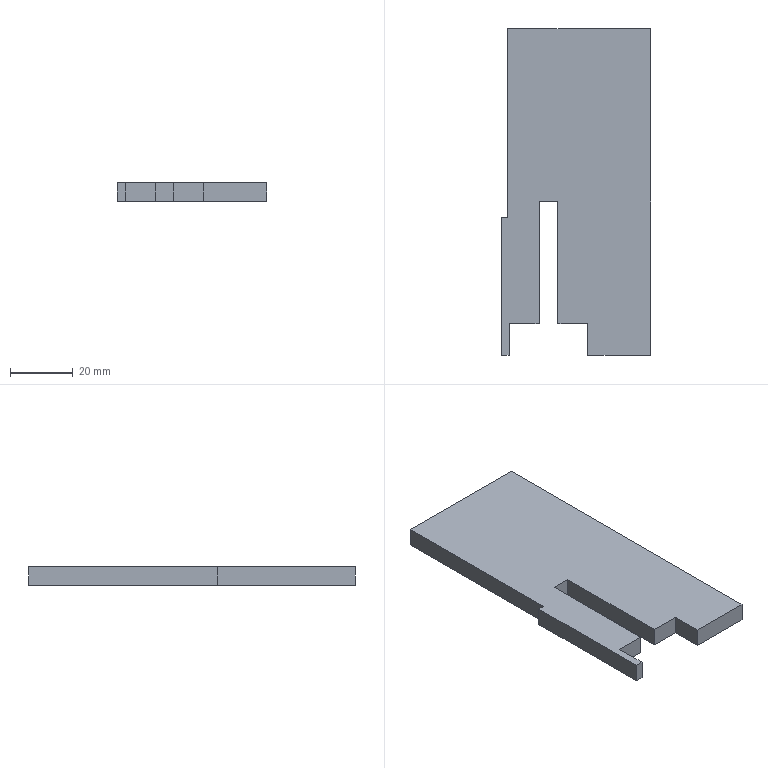Part | SolidWorks | features ICE 2, Extrusion 1 | 1 solid | 16 faces | box 47.5 x 103.96 x 6 mm | volume 26008 mm3 | plane 16
STEP:
#1=CARTESIAN_POINT('',(127.021,-23.465,0.));
#2=VERTEX_POINT('',#1);
#3=CARTESIAN_POINT('',(136.522,-23.465,0.));
#4=VERTEX_POINT('',#3);
#5=CARTESIAN_POINT('',(127.021,-23.465,0.));
#6=DIRECTION('',(1.,0.,0.));
#7=VECTOR('',#6,1000.);
#8=LINE('',#5,#7);
#9=EDGE_CURVE('',#2,#4,#8,.T.);
#10=ORIENTED_EDGE('',*,*,#9,.T.);
#11=CARTESIAN_POINT('',(136.522,-23.465,6.));
#12=VERTEX_POINT('',#11);
#13=CARTESIAN_POINT('',(136.522,-23.465,6.));
#14=DIRECTION('',(0.,0.,1.));
#15=VECTOR('',#14,1000.);
#16=LINE('',#13,#15);
#17=EDGE_CURVE('',#4,#12,#16,.T.);
#18=ORIENTED_EDGE('',*,*,#17,.T.);
#19=CARTESIAN_POINT('',(127.021,-23.465,6.));
#20=VERTEX_POINT('',#19);
#21=CARTESIAN_POINT('',(127.021,-23.465,6.));
#22=DIRECTION('',(1.,0.,0.));
#23=VECTOR('',#22,1000.);
#24=LINE('',#21,#23);
#25=EDGE_CURVE('',#20,#12,#24,.T.);
#26=ORIENTED_EDGE('',*,*,#25,.F.);
#27=CARTESIAN_POINT('',(127.021,-23.465,6.));
#28=DIRECTION('',(0.,0.,-1.));
#29=VECTOR('',#28,1000.);
#30=LINE('',#27,#29);
#31=EDGE_CURVE('',#20,#2,#30,.T.);
#32=ORIENTED_EDGE('',*,*,#31,.T.);
#33=EDGE_LOOP('',(#10,#18,#26,#32));
#34=FACE_OUTER_BOUND('',#33,.T.);
#35=CARTESIAN_POINT('',(127.021,-23.465,6.));
#36=DIRECTION('',(0.,1.,0.));
#37=DIRECTION('',(0.,0.,1.));
#38=AXIS2_PLACEMENT_3D('',#35,#36,#37);
#39=PLANE('',#38);
#40=ADVANCED_FACE('',(#34),#39,.F.);
#41=CARTESIAN_POINT('',(127.021,-33.445,0.));
#42=VERTEX_POINT('',#41);
#43=CARTESIAN_POINT('',(127.021,-33.445,0.));
#44=DIRECTION('',(0.,1.,0.));
#45=VECTOR('',#44,1000.);
#46=LINE('',#43,#45);
#47=EDGE_CURVE('',#42,#2,#46,.T.);
#48=ORIENTED_EDGE('',*,*,#47,.T.);
#49=ORIENTED_EDGE('',*,*,#31,.F.);
#50=CARTESIAN_POINT('',(127.021,-33.445,6.));
#51=VERTEX_POINT('',#50);
#52=CARTESIAN_POINT('',(127.021,-33.445,6.));
#53=DIRECTION('',(0.,1.,0.));
#54=VECTOR('',#53,1000.);
#55=LINE('',#52,#54);
#56=EDGE_CURVE('',#51,#20,#55,.T.);
#57=ORIENTED_EDGE('',*,*,#56,.F.);
#58=CARTESIAN_POINT('',(127.021,-33.445,6.));
#59=DIRECTION('',(0.,0.,-1.));
#60=VECTOR('',#59,1000.);
#61=LINE('',#58,#60);
#62=EDGE_CURVE('',#51,#42,#61,.T.);
#63=ORIENTED_EDGE('',*,*,#62,.T.);
#64=EDGE_LOOP('',(#48,#49,#57,#63));
#65=FACE_OUTER_BOUND('',#64,.T.);
#66=CARTESIAN_POINT('',(127.021,-33.445,6.));
#67=DIRECTION('',(-1.,0.,0.));
#68=DIRECTION('',(0.,0.,1.));
#69=AXIS2_PLACEMENT_3D('',#66,#67,#68);
#70=PLANE('',#69);
#71=ADVANCED_FACE('',(#65),#70,.F.);
#72=CARTESIAN_POINT('',(142.522,-23.465,6.));
#73=VERTEX_POINT('',#72);
#74=CARTESIAN_POINT('',(152.022,-23.465,6.));
#75=VERTEX_POINT('',#74);
#76=CARTESIAN_POINT('',(127.021,-23.465,6.));
#77=DIRECTION('',(1.,0.,0.));
#78=VECTOR('',#77,1000.);
#79=LINE('',#76,#78);
#80=EDGE_CURVE('',#73,#75,#79,.T.);
#81=ORIENTED_EDGE('',*,*,#80,.F.);
#82=CARTESIAN_POINT('',(142.522,-23.465,0.));
#83=VERTEX_POINT('',#82);
#84=CARTESIAN_POINT('',(142.522,-23.465,6.));
#85=DIRECTION('',(0.,0.,-1.));
#86=VECTOR('',#85,1000.);
#87=LINE('',#84,#86);
#88=EDGE_CURVE('',#73,#83,#87,.T.);
#89=ORIENTED_EDGE('',*,*,#88,.T.);
#90=CARTESIAN_POINT('',(152.022,-23.465,0.));
#91=VERTEX_POINT('',#90);
#92=CARTESIAN_POINT('',(127.021,-23.465,0.));
#93=DIRECTION('',(1.,0.,0.));
#94=VECTOR('',#93,1000.);
#95=LINE('',#92,#94);
#96=EDGE_CURVE('',#83,#91,#95,.T.);
#97=ORIENTED_EDGE('',*,*,#96,.T.);
#98=CARTESIAN_POINT('',(152.022,-23.465,6.));
#99=DIRECTION('',(0.,0.,-1.));
#100=VECTOR('',#99,1000.);
#101=LINE('',#98,#100);
#102=EDGE_CURVE('',#75,#91,#101,.T.);
#103=ORIENTED_EDGE('',*,*,#102,.F.);
#104=EDGE_LOOP('',(#81,#89,#97,#103));
#105=FACE_OUTER_BOUND('',#104,.T.);
#106=CARTESIAN_POINT('',(127.021,-23.465,6.));
#107=DIRECTION('',(0.,1.,0.));
#108=DIRECTION('',(0.,0.,1.));
#109=AXIS2_PLACEMENT_3D('',#106,#107,#108);
#110=PLANE('',#109);
#111=ADVANCED_FACE('',(#105),#110,.F.);
#112=CARTESIAN_POINT('',(152.022,-33.445,0.));
#113=VERTEX_POINT('',#112);
#114=CARTESIAN_POINT('',(152.022,-23.465,0.));
#115=DIRECTION('',(0.,-1.,0.));
#116=VECTOR('',#115,1000.);
#117=LINE('',#114,#116);
#118=EDGE_CURVE('',#91,#113,#117,.T.);
#119=ORIENTED_EDGE('',*,*,#118,.T.);
#120=CARTESIAN_POINT('',(152.022,-33.445,6.));
#121=VERTEX_POINT('',#120);
#122=CARTESIAN_POINT('',(152.022,-33.445,6.));
#123=DIRECTION('',(0.,0.,-1.));
#124=VECTOR('',#123,1000.);
#125=LINE('',#122,#124);
#126=EDGE_CURVE('',#121,#113,#125,.T.);
#127=ORIENTED_EDGE('',*,*,#126,.F.);
#128=CARTESIAN_POINT('',(152.022,-23.465,6.));
#129=DIRECTION('',(0.,-1.,0.));
#130=VECTOR('',#129,1000.);
#131=LINE('',#128,#130);
#132=EDGE_CURVE('',#75,#121,#131,.T.);
#133=ORIENTED_EDGE('',*,*,#132,.F.);
#134=ORIENTED_EDGE('',*,*,#102,.T.);
#135=EDGE_LOOP('',(#119,#127,#133,#134));
#136=FACE_OUTER_BOUND('',#135,.T.);
#137=CARTESIAN_POINT('',(152.022,-23.465,6.));
#138=DIRECTION('',(1.,0.,0.));
#139=DIRECTION('',(0.,0.,-1.));
#140=AXIS2_PLACEMENT_3D('',#137,#138,#139);
#141=PLANE('',#140);
#142=ADVANCED_FACE('',(#136),#141,.F.);
#143=CARTESIAN_POINT('',(172.022,-33.445,0.));
#144=VERTEX_POINT('',#143);
#145=CARTESIAN_POINT('',(152.022,-33.445,0.));
#146=DIRECTION('',(1.,0.,0.));
#147=VECTOR('',#146,1000.);
#148=LINE('',#145,#147);
#149=EDGE_CURVE('',#113,#144,#148,.T.);
#150=ORIENTED_EDGE('',*,*,#149,.T.);
#151=CARTESIAN_POINT('',(172.022,-33.445,6.));
#152=VERTEX_POINT('',#151);
#153=CARTESIAN_POINT('',(172.022,-33.445,6.));
#154=DIRECTION('',(0.,0.,-1.));
#155=VECTOR('',#154,1000.);
#156=LINE('',#153,#155);
#157=EDGE_CURVE('',#152,#144,#156,.T.);
#158=ORIENTED_EDGE('',*,*,#157,.F.);
#159=CARTESIAN_POINT('',(152.022,-33.445,6.));
#160=DIRECTION('',(1.,0.,0.));
#161=VECTOR('',#160,1000.);
#162=LINE('',#159,#161);
#163=EDGE_CURVE('',#121,#152,#162,.T.);
#164=ORIENTED_EDGE('',*,*,#163,.F.);
#165=ORIENTED_EDGE('',*,*,#126,.T.);
#166=EDGE_LOOP('',(#150,#158,#164,#165));
#167=FACE_OUTER_BOUND('',#166,.T.);
#168=CARTESIAN_POINT('',(152.022,-33.445,6.));
#169=DIRECTION('',(0.,1.,0.));
#170=DIRECTION('',(-1.,0.,0.));
#171=AXIS2_PLACEMENT_3D('',#168,#169,#170);
#172=PLANE('',#171);
#173=ADVANCED_FACE('',(#167),#172,.F.);
#174=CARTESIAN_POINT('',(172.022,70.515,0.));
#175=VERTEX_POINT('',#174);
#176=CARTESIAN_POINT('',(172.022,-33.445,0.));
#177=DIRECTION('',(0.,1.,0.));
#178=VECTOR('',#177,1000.);
#179=LINE('',#176,#178);
#180=EDGE_CURVE('',#144,#175,#179,.T.);
#181=ORIENTED_EDGE('',*,*,#180,.T.);
#182=CARTESIAN_POINT('',(172.022,70.515,6.));
#183=VERTEX_POINT('',#182);
#184=CARTESIAN_POINT('',(172.022,70.515,6.));
#185=DIRECTION('',(0.,0.,-1.));
#186=VECTOR('',#185,1000.);
#187=LINE('',#184,#186);
#188=EDGE_CURVE('',#183,#175,#187,.T.);
#189=ORIENTED_EDGE('',*,*,#188,.F.);
#190=CARTESIAN_POINT('',(172.022,-33.445,6.));
#191=DIRECTION('',(0.,1.,0.));
#192=VECTOR('',#191,1000.);
#193=LINE('',#190,#192);
#194=EDGE_CURVE('',#152,#183,#193,.T.);
#195=ORIENTED_EDGE('',*,*,#194,.F.);
#196=ORIENTED_EDGE('',*,*,#157,.T.);
#197=EDGE_LOOP('',(#181,#189,#195,#196));
#198=FACE_OUTER_BOUND('',#197,.T.);
#199=CARTESIAN_POINT('',(172.022,-33.445,6.));
#200=DIRECTION('',(-1.,0.,0.));
#201=DIRECTION('',(0.,0.,1.));
#202=AXIS2_PLACEMENT_3D('',#199,#200,#201);
#203=PLANE('',#202);
#204=ADVANCED_FACE('',(#198),#203,.F.);
#205=CARTESIAN_POINT('',(126.522,70.515,0.));
#206=VERTEX_POINT('',#205);
#207=CARTESIAN_POINT('',(172.022,70.515,0.));
#208=DIRECTION('',(-1.,0.,0.));
#209=VECTOR('',#208,1000.);
#210=LINE('',#207,#209);
#211=EDGE_CURVE('',#175,#206,#210,.T.);
#212=ORIENTED_EDGE('',*,*,#211,.T.);
#213=CARTESIAN_POINT('',(126.522,70.515,6.));
#214=VERTEX_POINT('',#213);
#215=CARTESIAN_POINT('',(126.522,70.515,0.));
#216=DIRECTION('',(0.,0.,1.));
#217=VECTOR('',#216,1000.);
#218=LINE('',#215,#217);
#219=EDGE_CURVE('',#206,#214,#218,.T.);
#220=ORIENTED_EDGE('',*,*,#219,.T.);
#221=CARTESIAN_POINT('',(172.022,70.515,6.));
#222=DIRECTION('',(-1.,0.,0.));
#223=VECTOR('',#222,1000.);
#224=LINE('',#221,#223);
#225=EDGE_CURVE('',#183,#214,#224,.T.);
#226=ORIENTED_EDGE('',*,*,#225,.F.);
#227=ORIENTED_EDGE('',*,*,#188,.T.);
#228=EDGE_LOOP('',(#212,#220,#226,#227));
#229=FACE_OUTER_BOUND('',#228,.T.);
#230=CARTESIAN_POINT('',(172.022,70.515,6.));
#231=DIRECTION('',(0.,-1.,0.));
#232=DIRECTION('',(1.,0.,0.));
#233=AXIS2_PLACEMENT_3D('',#230,#231,#232);
#234=PLANE('',#233);
#235=ADVANCED_FACE('',(#229),#234,.F.);
#236=CARTESIAN_POINT('',(124.522,-33.445,6.));
#237=VERTEX_POINT('',#236);
#238=CARTESIAN_POINT('',(127.021,-33.445,6.));
#239=DIRECTION('',(1.,0.,0.));
#240=VECTOR('',#239,1000.);
#241=LINE('',#238,#240);
#242=EDGE_CURVE('',#237,#51,#241,.T.);
#243=ORIENTED_EDGE('',*,*,#242,.F.);
#244=CARTESIAN_POINT('',(124.522,-33.445,0.));
#245=VERTEX_POINT('',#244);
#246=CARTESIAN_POINT('',(124.522,-33.445,6.));
#247=DIRECTION('',(0.,0.,-1.));
#248=VECTOR('',#247,1000.);
#249=LINE('',#246,#248);
#250=EDGE_CURVE('',#237,#245,#249,.T.);
#251=ORIENTED_EDGE('',*,*,#250,.T.);
#252=CARTESIAN_POINT('',(127.021,-33.445,0.));
#253=DIRECTION('',(1.,0.,0.));
#254=VECTOR('',#253,1000.);
#255=LINE('',#252,#254);
#256=EDGE_CURVE('',#245,#42,#255,.T.);
#257=ORIENTED_EDGE('',*,*,#256,.T.);
#258=ORIENTED_EDGE('',*,*,#62,.F.);
#259=EDGE_LOOP('',(#243,#251,#257,#258));
#260=FACE_OUTER_BOUND('',#259,.T.);
#261=CARTESIAN_POINT('',(127.021,-33.445,6.));
#262=DIRECTION('',(0.,1.,0.));
#263=DIRECTION('',(-1.,0.,0.));
#264=AXIS2_PLACEMENT_3D('',#261,#262,#263);
#265=PLANE('',#264);
#266=ADVANCED_FACE('',(#260),#265,.F.);
#267=CARTESIAN_POINT('',(124.522,10.515,6.));
#268=VERTEX_POINT('',#267);
#269=CARTESIAN_POINT('',(126.522,10.515,6.));
#270=VERTEX_POINT('',#269);
#271=CARTESIAN_POINT('',(124.522,10.515,6.));
#272=DIRECTION('',(1.,0.,0.));
#273=VECTOR('',#272,1000.);
#274=LINE('',#271,#273);
#275=EDGE_CURVE('',#268,#270,#274,.T.);
#276=ORIENTED_EDGE('',*,*,#275,.F.);
#277=CARTESIAN_POINT('',(124.522,10.515,6.));
#278=DIRECTION('',(0.,1.,0.));
#279=VECTOR('',#278,1000.);
#280=LINE('',#277,#279);
#281=EDGE_CURVE('',#237,#268,#280,.T.);
#282=ORIENTED_EDGE('',*,*,#281,.F.);
#283=ORIENTED_EDGE('',*,*,#242,.T.);
#284=ORIENTED_EDGE('',*,*,#56,.T.);
#285=ORIENTED_EDGE('',*,*,#25,.T.);
#286=CARTESIAN_POINT('',(136.522,15.515,6.));
#287=VERTEX_POINT('',#286);
#288=CARTESIAN_POINT('',(136.522,0.,6.));
#289=DIRECTION('',(0.,1.,0.));
#290=VECTOR('',#289,1000.);
#291=LINE('',#288,#290);
#292=EDGE_CURVE('',#12,#287,#291,.T.);
#293=ORIENTED_EDGE('',*,*,#292,.T.);
#294=CARTESIAN_POINT('',(142.522,15.515,6.));
#295=VERTEX_POINT('',#294);
#296=CARTESIAN_POINT('',(0.,15.515,6.));
#297=DIRECTION('',(1.,0.,0.));
#298=VECTOR('',#297,1000.);
#299=LINE('',#296,#298);
#300=EDGE_CURVE('',#287,#295,#299,.T.);
#301=ORIENTED_EDGE('',*,*,#300,.T.);
#302=CARTESIAN_POINT('',(142.522,0.,6.));
#303=DIRECTION('',(0.,-1.,0.));
#304=VECTOR('',#303,1000.);
#305=LINE('',#302,#304);
#306=EDGE_CURVE('',#295,#73,#305,.T.);
#307=ORIENTED_EDGE('',*,*,#306,.T.);
#308=ORIENTED_EDGE('',*,*,#80,.T.);
#309=ORIENTED_EDGE('',*,*,#132,.T.);
#310=ORIENTED_EDGE('',*,*,#163,.T.);
#311=ORIENTED_EDGE('',*,*,#194,.T.);
#312=ORIENTED_EDGE('',*,*,#225,.T.);
#313=CARTESIAN_POINT('',(126.522,10.515,6.));
#314=DIRECTION('',(0.,1.,0.));
#315=VECTOR('',#314,1000.);
#316=LINE('',#313,#315);
#317=EDGE_CURVE('',#270,#214,#316,.T.);
#318=ORIENTED_EDGE('',*,*,#317,.F.);
#319=EDGE_LOOP('',(#276,#282,#283,#284,#285,#293,#301,#307,#308,#309,#310,#311,#312,#318));
#320=FACE_OUTER_BOUND('',#319,.T.);
#321=CARTESIAN_POINT('',(0.,0.,6.));
#322=DIRECTION('',(0.,0.,-1.));
#323=DIRECTION('',(-1.,0.,0.));
#324=AXIS2_PLACEMENT_3D('',#321,#322,#323);
#325=PLANE('',#324);
#326=ADVANCED_FACE('',(#320),#325,.F.);
#327=CARTESIAN_POINT('',(124.522,10.515,0.));
#328=VERTEX_POINT('',#327);
#329=CARTESIAN_POINT('',(124.522,0.,0.));
#330=DIRECTION('',(0.,-1.,0.));
#331=VECTOR('',#330,1000.);
#332=LINE('',#329,#331);
#333=EDGE_CURVE('',#328,#245,#332,.T.);
#334=ORIENTED_EDGE('',*,*,#333,.F.);
#335=CARTESIAN_POINT('',(126.522,10.515,0.));
#336=VERTEX_POINT('',#335);
#337=CARTESIAN_POINT('',(124.522,10.515,0.));
#338=DIRECTION('',(1.,0.,0.));
#339=VECTOR('',#338,1000.);
#340=LINE('',#337,#339);
#341=EDGE_CURVE('',#328,#336,#340,.T.);
#342=ORIENTED_EDGE('',*,*,#341,.T.);
#343=CARTESIAN_POINT('',(126.522,10.515,0.));
#344=DIRECTION('',(0.,1.,0.));
#345=VECTOR('',#344,1000.);
#346=LINE('',#343,#345);
#347=EDGE_CURVE('',#336,#206,#346,.T.);
#348=ORIENTED_EDGE('',*,*,#347,.T.);
#349=ORIENTED_EDGE('',*,*,#211,.F.);
#350=ORIENTED_EDGE('',*,*,#180,.F.);
#351=ORIENTED_EDGE('',*,*,#149,.F.);
#352=ORIENTED_EDGE('',*,*,#118,.F.);
#353=ORIENTED_EDGE('',*,*,#96,.F.);
#354=CARTESIAN_POINT('',(142.522,15.515,0.));
#355=VERTEX_POINT('',#354);
#356=CARTESIAN_POINT('',(142.522,15.515,0.));
#357=DIRECTION('',(0.,-1.,0.));
#358=VECTOR('',#357,1000.);
#359=LINE('',#356,#358);
#360=EDGE_CURVE('',#355,#83,#359,.T.);
#361=ORIENTED_EDGE('',*,*,#360,.F.);
#362=CARTESIAN_POINT('',(136.522,15.515,0.));
#363=VERTEX_POINT('',#362);
#364=CARTESIAN_POINT('',(142.522,15.515,0.));
#365=DIRECTION('',(1.,0.,0.));
#366=VECTOR('',#365,1000.);
#367=LINE('',#364,#366);
#368=EDGE_CURVE('',#363,#355,#367,.T.);
#369=ORIENTED_EDGE('',*,*,#368,.F.);
#370=CARTESIAN_POINT('',(136.522,0.,0.));
#371=DIRECTION('',(0.,1.,0.));
#372=VECTOR('',#371,1000.);
#373=LINE('',#370,#372);
#374=EDGE_CURVE('',#4,#363,#373,.T.);
#375=ORIENTED_EDGE('',*,*,#374,.F.);
#376=ORIENTED_EDGE('',*,*,#9,.F.);
#377=ORIENTED_EDGE('',*,*,#47,.F.);
#378=ORIENTED_EDGE('',*,*,#256,.F.);
#379=EDGE_LOOP('',(#334,#342,#348,#349,#350,#351,#352,#353,#361,#369,#375,#376,#377,#378));
#380=FACE_OUTER_BOUND('',#379,.T.);
#381=CARTESIAN_POINT('',(0.,0.,0.));
#382=DIRECTION('',(0.,0.,-1.));
#383=DIRECTION('',(-1.,0.,0.));
#384=AXIS2_PLACEMENT_3D('',#381,#382,#383);
#385=PLANE('',#384);
#386=ADVANCED_FACE('',(#380),#385,.T.);
#387=CARTESIAN_POINT('',(136.522,15.515,10.));
#388=DIRECTION('',(0.,0.,-1.));
#389=VECTOR('',#388,1000.);
#390=LINE('',#387,#389);
#391=EDGE_CURVE('',#287,#363,#390,.T.);
#392=ORIENTED_EDGE('',*,*,#391,.T.);
#393=ORIENTED_EDGE('',*,*,#368,.T.);
#394=CARTESIAN_POINT('',(142.522,15.515,10.));
#395=DIRECTION('',(0.,0.,-1.));
#396=VECTOR('',#395,1000.);
#397=LINE('',#394,#396);
#398=EDGE_CURVE('',#295,#355,#397,.T.);
#399=ORIENTED_EDGE('',*,*,#398,.F.);
#400=ORIENTED_EDGE('',*,*,#300,.F.);
#401=EDGE_LOOP('',(#392,#393,#399,#400));
#402=FACE_OUTER_BOUND('',#401,.T.);
#403=CARTESIAN_POINT('',(142.522,15.515,10.));
#404=DIRECTION('',(0.,1.,0.));
#405=DIRECTION('',(0.,0.,1.));
#406=AXIS2_PLACEMENT_3D('',#403,#404,#405);
#407=PLANE('',#406);
#408=ADVANCED_FACE('',(#402),#407,.F.);
#409=ORIENTED_EDGE('',*,*,#374,.T.);
#410=ORIENTED_EDGE('',*,*,#391,.F.);
#411=ORIENTED_EDGE('',*,*,#292,.F.);
#412=ORIENTED_EDGE('',*,*,#17,.F.);
#413=EDGE_LOOP('',(#409,#410,#411,#412));
#414=FACE_OUTER_BOUND('',#413,.T.);
#415=CARTESIAN_POINT('',(136.522,15.515,10.));
#416=DIRECTION('',(-1.,0.,0.));
#417=DIRECTION('',(0.,0.,1.));
#418=AXIS2_PLACEMENT_3D('',#415,#416,#417);
#419=PLANE('',#418);
#420=ADVANCED_FACE('',(#414),#419,.F.);
#421=ORIENTED_EDGE('',*,*,#306,.F.);
#422=ORIENTED_EDGE('',*,*,#398,.T.);
#423=ORIENTED_EDGE('',*,*,#360,.T.);
#424=ORIENTED_EDGE('',*,*,#88,.F.);
#425=EDGE_LOOP('',(#421,#422,#423,#424));
#426=FACE_OUTER_BOUND('',#425,.T.);
#427=CARTESIAN_POINT('',(142.522,15.515,10.));
#428=DIRECTION('',(1.,0.,0.));
#429=DIRECTION('',(0.,0.,-1.));
#430=AXIS2_PLACEMENT_3D('',#427,#428,#429);
#431=PLANE('',#430);
#432=ADVANCED_FACE('',(#426),#431,.F.);
#433=ORIENTED_EDGE('',*,*,#281,.T.);
#434=CARTESIAN_POINT('',(124.522,10.515,0.));
#435=DIRECTION('',(0.,0.,1.));
#436=VECTOR('',#435,1000.);
#437=LINE('',#434,#436);
#438=EDGE_CURVE('',#328,#268,#437,.T.);
#439=ORIENTED_EDGE('',*,*,#438,.F.);
#440=ORIENTED_EDGE('',*,*,#333,.T.);
#441=ORIENTED_EDGE('',*,*,#250,.F.);
#442=EDGE_LOOP('',(#433,#439,#440,#441));
#443=FACE_OUTER_BOUND('',#442,.T.);
#444=CARTESIAN_POINT('',(124.522,10.515,0.));
#445=DIRECTION('',(1.,0.,0.));
#446=DIRECTION('',(0.,1.,0.));
#447=AXIS2_PLACEMENT_3D('',#444,#445,#446);
#448=PLANE('',#447);
#449=ADVANCED_FACE('',(#443),#448,.F.);
#450=ORIENTED_EDGE('',*,*,#317,.T.);
#451=ORIENTED_EDGE('',*,*,#219,.F.);
#452=ORIENTED_EDGE('',*,*,#347,.F.);
#453=CARTESIAN_POINT('',(126.522,10.515,0.));
#454=DIRECTION('',(0.,0.,1.));
#455=VECTOR('',#454,1000.);
#456=LINE('',#453,#455);
#457=EDGE_CURVE('',#336,#270,#456,.T.);
#458=ORIENTED_EDGE('',*,*,#457,.T.);
#459=EDGE_LOOP('',(#450,#451,#452,#458));
#460=FACE_OUTER_BOUND('',#459,.T.);
#461=CARTESIAN_POINT('',(126.522,10.515,0.));
#462=DIRECTION('',(1.,0.,0.));
#463=DIRECTION('',(0.,0.,-1.));
#464=AXIS2_PLACEMENT_3D('',#461,#462,#463);
#465=PLANE('',#464);
#466=ADVANCED_FACE('',(#460),#465,.F.);
#467=ORIENTED_EDGE('',*,*,#275,.T.);
#468=ORIENTED_EDGE('',*,*,#457,.F.);
#469=ORIENTED_EDGE('',*,*,#341,.F.);
#470=ORIENTED_EDGE('',*,*,#438,.T.);
#471=EDGE_LOOP('',(#467,#468,#469,#470));
#472=FACE_OUTER_BOUND('',#471,.T.);
#473=CARTESIAN_POINT('',(124.522,10.515,0.));
#474=DIRECTION('',(0.,-1.,0.));
#475=DIRECTION('',(0.,0.,-1.));
#476=AXIS2_PLACEMENT_3D('',#473,#474,#475);
#477=PLANE('',#476);
#478=ADVANCED_FACE('',(#472),#477,.F.);
#479=CLOSED_SHELL('',(#40,#71,#111,#142,#173,#204,#235,#266,#326,#386,#408,#420,#432,#449,#466,#478));
#480=MANIFOLD_SOLID_BREP('',#479);
#481=CARTESIAN_POINT('',(0.,0.,0.));
#482=DIRECTION('',(0.,0.,1.));
#483=DIRECTION('',(1.,0.,0.));
#484=AXIS2_PLACEMENT_3D('',#481,#482,#483);
#485=(LENGTH_UNIT()NAMED_UNIT(*)SI_UNIT(.MILLI.,.METRE.));
#486=UNCERTAINTY_MEASURE_WITH_UNIT(LENGTH_MEASURE(0.00001),#485,'','');
#487=(NAMED_UNIT(*)PLANE_ANGLE_UNIT()SI_UNIT($,.RADIAN.));
#488=(NAMED_UNIT(*)SI_UNIT($,.STERADIAN.)SOLID_ANGLE_UNIT());
#489=(GEOMETRIC_REPRESENTATION_CONTEXT(3)GLOBAL_UNCERTAINTY_ASSIGNED_CONTEXT((#486))GLOBAL_UNIT_ASSIGNED_CONTEXT((#485,#487,#488))REPRESENTATION_CONTEXT('',''));
#490=ADVANCED_BREP_SHAPE_REPRESENTATION('',(#480,#484),#489);